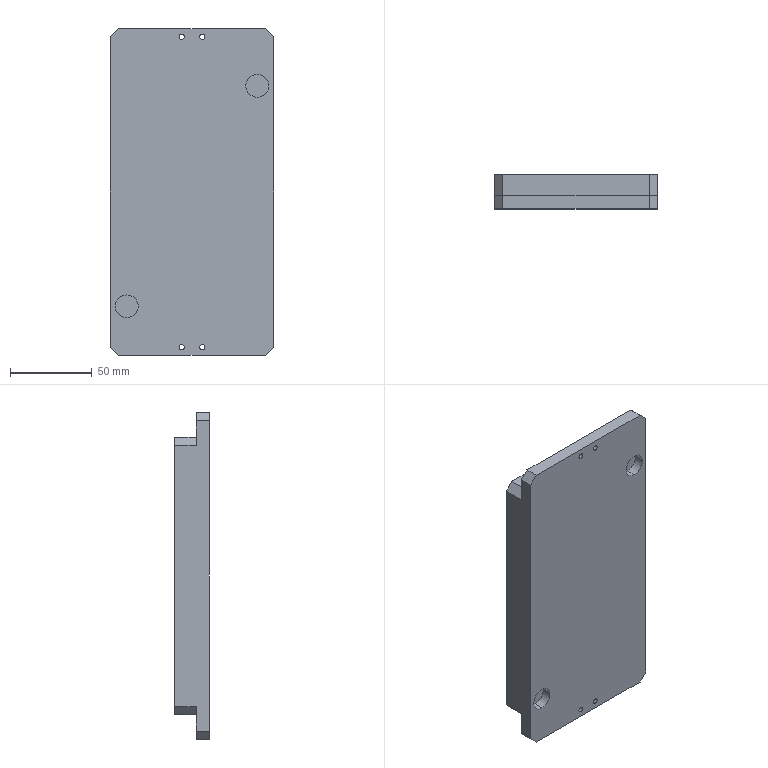Part | STEP file | ZHIJUBAN-1_1-2 | 1 solid | 86 faces | box 100 x 21 x 200 mm | volume 345878 mm3 | plane 42 | cylinder 38 | spline 6 | commonest cylinder face diameters 4 x20 3.2 x8 16 x6 14 x4